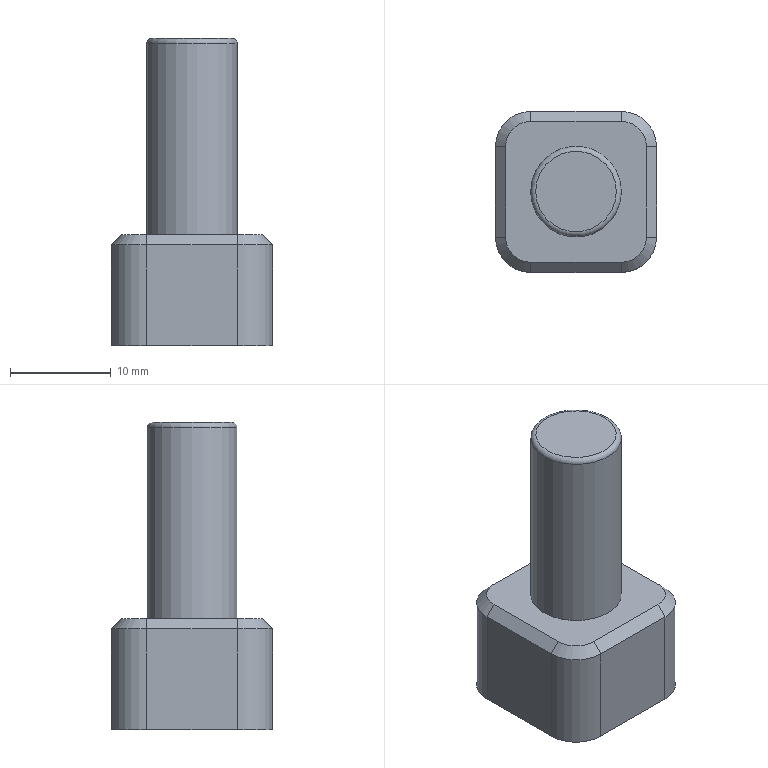NC program | NX | posted with a generic post | part box 16 x 16 x 30.5 mm
Whole program:
N10 G17 G21 G94 G90
(DYNAMIC_ROUGH_COPY , TOOL : D12-36-D12-75-3T_ROUGH)
N12 T01 M6
N14 G54
N16 G17 G0 G90 X-22.033 Y-0.845 S6500 M3
N18 G43 Z20. H1
N20 Z0.6
N22 G94 G1 X-22.008 Y-0.844 Z0.444 F3000.
N24 X-21.983 Y-0.842 Z0.382
N26 X-21.958 Y-0.841 Z0.337
N28 X-21.933 Y-0.84 Z0.3
N30 X-21.908 Y-0.839 Z0.269
N32 X-21.883 Y-0.838 Z0.243
N34 X-21.858 Y-0.837 Z0.22
N36 X-21.833 Y-0.836 Z0.2
N38 X-21.808 Y-0.834 Z0.182
N40 X-21.783 Y-0.833 Z0.167
N42 X-21.758 Y-0.832 Z0.153
N44 X-21.733 Y-0.831 Z0.142
N46 X-21.708 Y-0.83 Z0.132
N48 X-21.683 Y-0.829 Z0.123
N50 X-21.658 Y-0.828 Z0.116
N52 X-21.633 Y-0.826 Z0.11
N54 X-21.608 Y-0.825 Z0.106
N56 X-21.583 Y-0.824 Z0.103
N58 X-21.558 Y-0.823 Z0.101
N60 X-21.533 Y-0.822 Z0.1
N62 X-19.567 Y-0.731
N64 G3 X-18.516 Y-0.013 R1.213
N66 X-17.796 Y2.548 R26.44
N68 G2 X-14.682 Y9.79 R22.304
N70 X15.89 Y7.578 R17.655
N72 X-17.156 Y-3.877 R-17.598
N74 X-16.96 Y2.291 R16.027
N76 X-10.775 Y12.812 R18.478
N78 X5.988 Y-15.6 R-16.722
N80 X-15.599 Y-5.935 R16.644
N82 X-15.921 Y2.851 R15.645
N84 X-6.248 Y14.527 R16.805
N86 X-12.9 Y-9.106 R-15.796
N88 X-15.231 Y1.586 R14.498
N90 X-4.727 Y14.103 R15.728
N92 X-8.215 Y-12.365 R-14.852
N94 X-14.191 Y1.945 R13.852
N96 X-1.881 Y13.76 R14.56
N98 X-7.916 Y-11.369 R-13.865
N100 X-13.024 Y2.589 R13.075
N102 X0.607 Y12.84 R13.404
N104 X-5.585 Y-11.531 R-12.83
N106 X-11.663 Y3.452 R12.161
N108 X2.819 Y11.407 R12.215
N110 X-3.445 Y-11.179 R-11.724
N112 X-9.355 Y5.579 R11.131
N114 X6.089 Y8.593 R10.889
N116 X-1.784 Y-10.314 R10.5
N118 X-2.47 Y8.994 R9.884
N120 X8.968 Y-1.523 R9.281
N122 X-1.72 Y-8.83 R8.965
N124 X-5.697 Y5.5 R8.392
N126 X5.655 Y4.741 R7.773
N128 X4.068 Y-5.869 R7.266
N130 X-4.732 Y-4.364 R6.462
N132 X-5.055 Y1.865 R5.601
N134 X-2.804 Y3.819 R5.848
N136 G1 X-2.782 Y3.832 Z0.101
N138 X-2.761 Y3.844 Z0.103
N140 X-2.739 Y3.856 Z0.106
N142 X-2.717 Y3.869 Z0.11
N144 X-2.696 Y3.881 Z0.116
N146 X-2.674 Y3.894 Z0.123
N148 X-2.652 Y3.906 Z0.132
N150 X-2.63 Y3.919 Z0.142
N152 X-2.609 Y3.931 Z0.153
N154 X-2.587 Y3.944 Z0.167
N156 X-2.565 Y3.956 Z0.182
N158 X-2.544 Y3.968 Z0.2
N160 X-2.522 Y3.981 Z0.22
N162 X-2.5 Y3.993 Z0.243
N164 X-2.479 Y4.006 Z0.269
N166 X-2.457 Y4.018 Z0.3
N168 X-2.435 Y4.031 Z0.337
N170 X-2.414 Y4.043 Z0.382
N172 X-2.392 Y4.055 Z0.444
N174 X-2.37 Y4.068 Z0.6
N176 G0 Z20.
N178 M5
(FLOOR_WALL_1 , TOOL : D12-36-D12-120-3T_FINISH)
N180 T02 M6
N182 G54
N184 G17 G0 G90 X-16.99 Y4.999 S4500 M3
N186 G43 Z20. H2
N188 Z3.
N190 G94 G1 Z0. F1000.
N192 X-13.987
N194 X13.987 Y5.001
N196 G2 X14. Y4.5 R9.5
N198 G1 Y-3.199
N200 X-14. Y-3.201
N202 X-17.
N204 Z3.
N206 G0 Z20.
N208 M5
(PLANAR_MILL_2 , TOOL : CHAMFER_D8-90DEG)
N210 T03 M6
N212 G54
N214 G17 G0 G90 X-10.5 Y-1. S4500 M3
N216 G43 Z20. H3
N218 Z0.5
N220 G94 G1 Z-1.5 F1000.
N222 G3 X-9.5 Y0. R1.
N224 G1 Y4.5
N226 G2 X-4.5 Y9.5 R5.
N228 G1 X4.5
N230 G2 X9.5 Y4.5 R5.
N232 G1 Y-4.5
N234 G2 X4.5 Y-9.5 R5.
N236 G1 X-4.5
N238 G2 X-9.5 Y-4.5 R5.
N240 G1 Y0.
N242 G3 X-10.5 Y1. R1.
N244 G1 Z0.5
N246 G0 Z20.
N248 M5
N250 M2